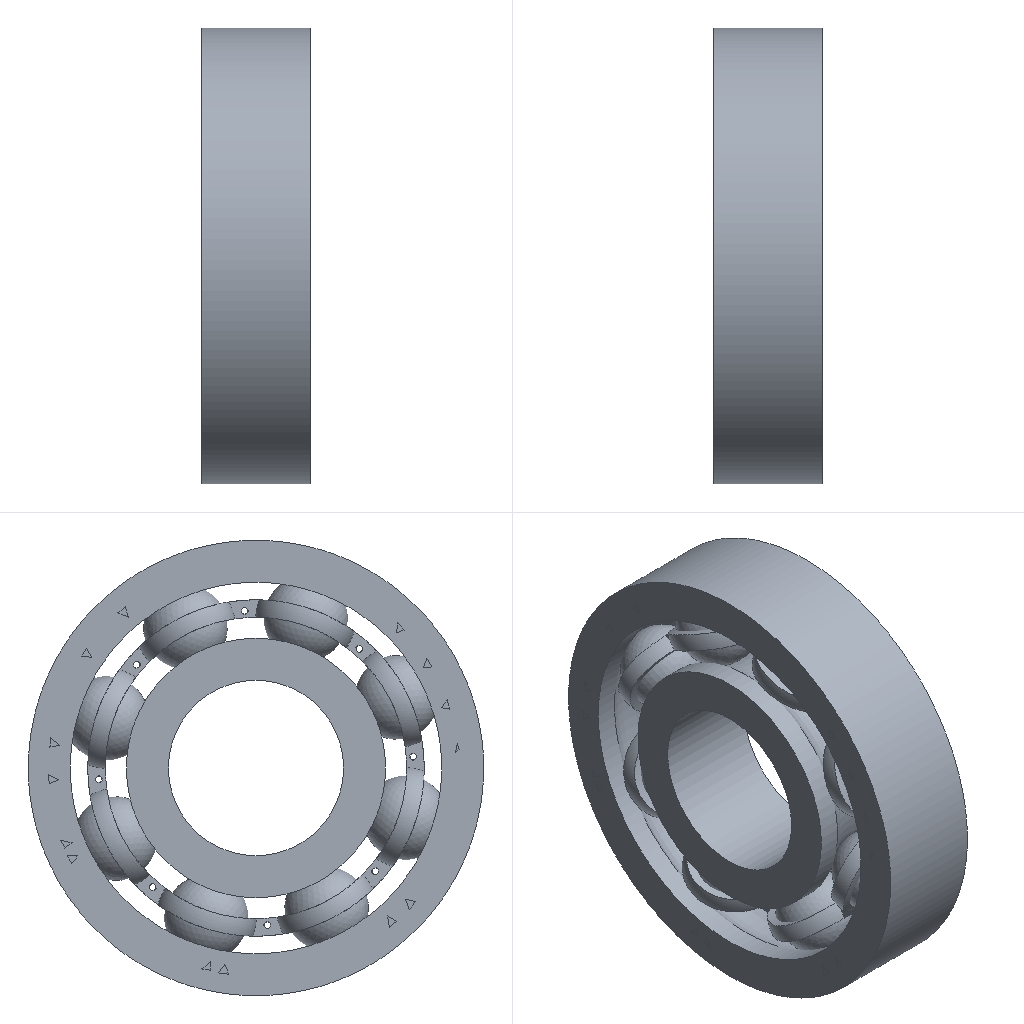Simulation study | ansys workbench
Set-up summary:
category,name,step,type,value,unit,region
solver,ansys_workbench
units,SI m-kg-s (Pa),,stated,"/units,MKS"
analysis,LS1,,static
load_step,LS1,LS1,static,nsubst=1; time=1
mesh,nodes,,,291728
mesh,elements,,,199572
element_type,SOLID187,,,151094
element_type,TARGE170,,,18876
element_type,CONTA174,,,18876
element_type,SOLID186,,,10416
element_type,SURF154,,,310
material,Structural Steel,,E,2e+11,Pa
material,Structural Steel,,nu,0.3
material,Structural Steel,,density,7850,kg m^-3
material,Structural Steel,,conductivity,60.5,W m^-1 C^-1
material,Structural Steel,,specific_heat,434,J kg^-1 C^-1
material,Structural Steel,,cte,1.2e-05,C^-1
material,Structural Steel,,permeability,10000
material,Structural Steel,,resistivity,1.7e-07,kg m^3 A^-2 s^-3
load,Define Force Using Surface Effect Elements,LS1,surface-effect pres face 1,-17113.4,,SURF154 #79
bc,Fixed Supports,model,fixed,[dofs=ALL],,_FIXEDSU
contact,Contact Region,,bonded (always),element=CONTA174
contact,Contact Region 2,,bonded (always),element=CONTA174
contact,Contact Region 3,,bonded (always),element=CONTA174
contact,Contact Region 4,,bonded (always),element=CONTA174
contact,Contact Region 5,,bonded (always),element=CONTA174
contact,Contact Region 6,,bonded (always),element=CONTA174
contact,Contact Region 7,,bonded (always),element=CONTA174
contact,Contact Region 8,,bonded (always),element=CONTA174
contact,Contact Region 9,,bonded (always),element=CONTA174
contact,Contact Region 10,,bonded (always),element=CONTA174
contact,Contact Region 11,,bonded (always),element=CONTA174
contact,Contact Region 12,,bonded (always),element=CONTA174
contact,Contact Region 21,,bonded (always),element=CONTA174
contact,Contact Region 22,,bonded (always),element=CONTA174
contact,Contact Region 23,,bonded (always),element=CONTA174
contact,Contact Region 24,,bonded (always),element=CONTA174
contact,Contact Region 25,,bonded (always),element=CONTA174
contact,Contact Region 26,,bonded (always),element=CONTA174
contact,Contact Region 27,,bonded (always),element=CONTA174
contact,Contact Region 28,,bonded (always),element=CONTA174
contact,Contact Region 29,,bonded (always),element=CONTA174
contact,Contact Region 30,,bonded (always),element=CONTA174
contact,Contact Region 31,,bonded (always),element=CONTA174
contact,Contact Region 32,,bonded (always),element=CONTA174
contact,Contact Region 33,,bonded (always),element=CONTA174
contact,Contact Region 34,,bonded (always),element=CONTA174
contact,Contact Region 35,,bonded (always),element=CONTA174
contact,Contact Region 36,,bonded (always),element=CONTA174
contact,Contact Region 39,,bonded (always),element=CONTA174
contact,Contact Region 40,,bonded (always),element=CONTA174
contact,Contact Region 41,,bonded (always),element=CONTA174
contact,Contact Region 42,,bonded (always),element=CONTA174
contact,Contact Region 43,,bonded (always),element=CONTA174
named_set,_FIXEDSU,,node,1910
Ansys APDL input file, long lists of numbers shortened:
/batch
/config,noeldb,1     ! force off writing results to database
*get,_wallstrt,active,,time,wall
! ANSYS input file written by Workbench version 2024 R2
! File used for geometry attach:
/title,wbnew--____ (A5)
! ****** Begin Custom Load Command Snippet ******
/COM, ACT Extensions:
/COM,     LSDYNA, 2024.2
/COM,/COM,     ANSYSMotion, 2024.2
/COM,
! ****** End   Custom Load Command Snippet ******
*DIM,_wb_ProjectScratch_dir,string,248
_wb_ProjectScratch_dir(1) = ''
*DIM,_wb_SolverFiles_dir,string,248
_wb_SolverFiles_dir(1) = ''
*DIM,_wb_userfiles_dir,string,248
_wb_userfiles_dir(1) = ''
/com,--- Data in consistent MKS units. See Solving Units in the help system for more information.
/units,MKS
/nopr
/wb,file,start              !  signify a WB generated input file
/prep7
! Turn off shape checking because checks already performed inside WB mesher.
! See help system for more information.
SHPP,OFF,,NOWARN
/nolist
etcon,set             ! allow ANSYS to choose best KEYOP's for 180x elements, resets any applicable keyopt to MAPDL defaults
/com,*********** Nodes for the whole assembly ***********
nblock,3,,320900
(1i9,3e20.9e3)
        1     7.105415696E-02    -1.310212572E-01    -3.338176666E-02
! (291727 more lines like these left out)
-1
/wb,elem,start            !  set before creation of elements
/com,*********** Elements for Body 1 'ball 3|Revolve1' ***********
et,1,187
eblock,19,solid,,8093
(19i9)
        1        1        1        1        0        0        0        0       10        0        1      749      951     1669     1661     6914     8412     6923     6922
! (16185 more lines like these left out)
-1
/com,*********** Elements for Body 2 'cage 4|CirPattern2' ***********
et,2,187
eblock,19,solid,,43175
(19i9)
        2        2        2        2        0        0        0        0       10        0     8094    18166    18230    18232    23065    62092    62544    62093    62097
! (86349 more lines like these left out)
-1
/com,*********** Elements for Body 3 'inner ring 2|Revolve1' ***********
et,3,186
keyo,3,2,1          ! set full integration on SOLID186
eblock,19,solid,,3720
(19i9)
        3        3        3        3        0        0        0        0       20        0    51269    84215    84416    84251    84417    87104    86903    87068    86902
! (7439 more lines like these left out)
-1
/com,*********** Elements for Body 4 'outer ring 1|Revolve2' ***********
et,4,186
keyo,4,2,1          ! set full integration on SOLID186
eblock,19,solid,,6696
(19i9)
        4        4        4        4        0        0        0        0       20        0    54989   102514   102900   102901   102546   107625   107239   107238   107593
! (13391 more lines like these left out)
-1
/com,*********** Elements for Body 5 'ball 3|Revolve1[2]' ***********
et,5,187
eblock,19,solid,,8093
(19i9)
        5        5        5        5        0        0        0        0       10        0    61685   136204   136406   137124   137116   142369   143867   142378   142377
! (16185 more lines like these left out)
-1
/com,*********** Elements for Body 6 'ball 3|Revolve1[3]' ***********
et,6,187
eblock,19,solid,,8093
(19i9)
        6        6        6        6        0        0        0        0       10        0    69778   148217   148419   149137   149129   154382   155880   154391   154390
! (16185 more lines like these left out)
-1
/com,*********** Elements for Body 7 'ball 3|Revolve1[4]' ***********
et,7,187
eblock,19,solid,,8093
(19i9)
        7        7        7        7        0        0        0        0       10        0    77871   160230   160432   161150   161142   166395   167893   166404   166403
! (16185 more lines like these left out)
-1
/com,*********** Elements for Body 8 'ball 3|Revolve1[5]' ***********
et,8,187
eblock,19,solid,,8093
(19i9)
        8        8        8        8        0        0        0        0       10        0    85964   172243   172445   173163   173155   178408   179906   178417   178416
! (16185 more lines like these left out)
-1
/com,*********** Elements for Body 9 'ball 3|Revolve1[6]' ***********
et,9,187
eblock,19,solid,,8093
(19i9)
        9        9        9        9        0        0        0        0       10        0    94057   184256   184458   185176   185168   190421   191919   190430   190429
! (16185 more lines like these left out)
-1
! (2 more sections like these left out)
/com,*********** Elements for Body 12 'cage 4|CirPattern2[2]' ***********
et,12,187
eblock,19,solid,,43175
(19i9)
       12       12       12       12        0        0        0        0       10        0   118336   225699   225763   225765   230598   269625   270077   269626   269630
! (86349 more lines like these left out)
-1
/wb,elem,end               !  done creating elements
/com,*********** Send User Defined Coordinate System(s) ***********
csys,0
toffst,273.15,      ! Temperature offset from absolute zero
/com,*********** Set Reference Temperature ***********
tref,22.
/wb,mat,start              !  starting to send materials
/com,*********** Send Materials ***********
Temperature = 'TEMP' ! Temperature
MP,DENS,1,7850,	! kg m^-3
MP,ALPX,1,1.2e-05,	! C^-1
MP,C,1,434,	! J kg^-1 C^-1
MP,KXX,1,60.5,	! W m^-1 C^-1
MP,RSVX,1,1.7e-07,	! kg m^3 A^-2 s^-3
MP,EX,1,200000000000,	! Pa
MP,NUXY,1,0.3,
MP,MURX,1,10000,
Temperature = 'TEMP' ! Temperature
MP,DENS,2,7850,	! kg m^-3
MP,ALPX,2,1.2e-05,	! C^-1
MP,C,2,434,	! J kg^-1 C^-1
MP,KXX,2,60.5,	! W m^-1 C^-1
MP,RSVX,2,1.7e-07,	! kg m^3 A^-2 s^-3
MP,EX,2,200000000000,	! Pa
MP,NUXY,2,0.3,
MP,MURX,2,10000,
Temperature = 'TEMP' ! Temperature
MP,DENS,3,7850,	! kg m^-3
MP,ALPX,3,1.2e-05,	! C^-1
MP,C,3,434,	! J kg^-1 C^-1
MP,KXX,3,60.5,	! W m^-1 C^-1
MP,RSVX,3,1.7e-07,	! kg m^3 A^-2 s^-3
MP,EX,3,200000000000,	! Pa
MP,NUXY,3,0.3,
MP,MURX,3,10000,
Temperature = 'TEMP' ! Temperature
MP,DENS,4,7850,	! kg m^-3
MP,ALPX,4,1.2e-05,	! C^-1
MP,C,4,434,	! J kg^-1 C^-1
MP,KXX,4,60.5,	! W m^-1 C^-1
MP,RSVX,4,1.7e-07,	! kg m^3 A^-2 s^-3
MP,EX,4,200000000000,	! Pa
MP,NUXY,4,0.3,
MP,MURX,4,10000,
Temperature = 'TEMP' ! Temperature
MP,DENS,5,7850,	! kg m^-3
MP,ALPX,5,1.2e-05,	! C^-1
MP,C,5,434,	! J kg^-1 C^-1
MP,KXX,5,60.5,	! W m^-1 C^-1
MP,RSVX,5,1.7e-07,	! kg m^3 A^-2 s^-3
MP,EX,5,200000000000,	! Pa
MP,NUXY,5,0.3,
MP,MURX,5,10000,
Temperature = 'TEMP' ! Temperature
MP,DENS,6,7850,	! kg m^-3
MP,ALPX,6,1.2e-05,	! C^-1
MP,C,6,434,	! J kg^-1 C^-1
MP,KXX,6,60.5,	! W m^-1 C^-1
MP,RSVX,6,1.7e-07,	! kg m^3 A^-2 s^-3
MP,EX,6,200000000000,	! Pa
MP,NUXY,6,0.3,
MP,MURX,6,10000,
Temperature = 'TEMP' ! Temperature
MP,DENS,7,7850,	! kg m^-3
MP,ALPX,7,1.2e-05,	! C^-1
MP,C,7,434,	! J kg^-1 C^-1
MP,KXX,7,60.5,	! W m^-1 C^-1
MP,RSVX,7,1.7e-07,	! kg m^3 A^-2 s^-3
MP,EX,7,200000000000,	! Pa
MP,NUXY,7,0.3,
MP,MURX,7,10000,
Temperature = 'TEMP' ! Temperature
MP,DENS,8,7850,	! kg m^-3
MP,ALPX,8,1.2e-05,	! C^-1
MP,C,8,434,	! J kg^-1 C^-1
MP,KXX,8,60.5,	! W m^-1 C^-1
MP,RSVX,8,1.7e-07,	! kg m^3 A^-2 s^-3
MP,EX,8,200000000000,	! Pa
MP,NUXY,8,0.3,
MP,MURX,8,10000,
Temperature = 'TEMP' ! Temperature
MP,DENS,9,7850,	! kg m^-3
MP,ALPX,9,1.2e-05,	! C^-1
MP,C,9,434,	! J kg^-1 C^-1
MP,KXX,9,60.5,	! W m^-1 C^-1
MP,RSVX,9,1.7e-07,	! kg m^3 A^-2 s^-3
MP,EX,9,200000000000,	! Pa
MP,NUXY,9,0.3,
MP,MURX,9,10000,
Temperature = 'TEMP' ! Temperature
MP,DENS,10,7850,	! kg m^-3
MP,ALPX,10,1.2e-05,	! C^-1
MP,C,10,434,	! J kg^-1 C^-1
MP,KXX,10,60.5,	! W m^-1 C^-1
MP,RSVX,10,1.7e-07,	! kg m^3 A^-2 s^-3
MP,EX,10,200000000000,	! Pa
MP,NUXY,10,0.3,
MP,MURX,10,10000,
Temperature = 'TEMP' ! Temperature
MP,DENS,11,7850,	! kg m^-3
MP,ALPX,11,1.2e-05,	! C^-1
MP,C,11,434,	! J kg^-1 C^-1
MP,KXX,11,60.5,	! W m^-1 C^-1
MP,RSVX,11,1.7e-07,	! kg m^3 A^-2 s^-3
MP,EX,11,200000000000,	! Pa
MP,NUXY,11,0.3,
MP,MURX,11,10000,
Temperature = 'TEMP' ! Temperature
MP,DENS,12,7850,	! kg m^-3
MP,ALPX,12,1.2e-05,	! C^-1
MP,C,12,434,	! J kg^-1 C^-1
MP,KXX,12,60.5,	! W m^-1 C^-1
MP,RSVX,12,1.7e-07,	! kg m^3 A^-2 s^-3
MP,EX,12,200000000000,	! Pa
MP,NUXY,12,0.3,
MP,MURX,12,10000,
/wb,mat,end                !  done sending materials
!************************* Model Summary ********************
!ball 3|Revolve1,	ç»æé¢,	matid,	1
!cage 4|CirPattern2,	ç»æé¢,	matid,	2
!inner ring 2|Revolve1,	ç»æé¢,	matid,	3
!outer ring 1|Revolve2,	ç»æé¢,	matid,	4
!ball 3|Revolve1[2],	ç»æé¢,	matid,	5
!ball 3|Revolve1[3],	ç»æé¢,	matid,	6
!ball 3|Revolve1[4],	ç»æé¢,	matid,	7
!ball 3|Revolve1[5],	ç»æé¢,	matid,	8
!ball 3|Revolve1[6],	ç»æé¢,	matid,	9
!ball 3|Revolve1[7],	ç»æé¢,	matid,	10
!ball 3|Revolve1[8],	ç»æé¢,	matid,	11
!cage 4|CirPattern2[2],	ç»æé¢,	matid,	12
!************************* End Model Summary ********************
! get the diagonal of the bounding box. Needed later for other things
*get,_xmin,node,,mnloc,x
*get,_ymin,node,,mnloc,y
*get,_zmin,node,,mnloc,z
*get,_xmax,node,,mxloc,x
*get,_ymax,node,,mxloc,y
*get,_zmax,node,,mxloc,z
_ASMDIAG=(_xmax-_xmin)*(_xmax-_xmin)+(_ymax-_ymin)*(_ymax-_ymin)+(_zmax-_zmin)*(_zmax-_zmin)
_ASMDIAG=SQRT(_ASMDIAG)
/wb,contact,start          !  starting to send contact
/com,*********** Create Contact "½Ó´¥ÇøÓò" ***********
/com,            Real Constant Set For Above Contact Is 14 & 13
*set,tid,14
*set,cid,13
r,tid
r,cid
et,tid,170
et,cid,174
eblock,10,,,275
(15i9)
   204739       14       14       14        0       36       37      315      315     1973     1985      315     1976
! (274 more lines like these left out)
-1
eblock,10,,,275
(15i9)
   205014       13       13       13        0       36       37      315      315     1973     1985      315     1976
! (274 more lines like these left out)
-1
eblock,10,,,440
(15i9)
   205289       13       14       13        0    13834    13833    18365    18365    34711    34715    18365    34721
! (439 more lines like these left out)
-1
eblock,10,,,440
(15i9)
   205729       14       13       14        0    13834    13833    18365    18365    34711    34715    18365    34721
! (439 more lines like these left out)
-1
keyo,cid,8,2               ! auto create asymmetric contact (from Program Controlled setting)
keyo,cid,10,0              ! adjust contact stiffness each NR iteration (from Program Controlled setting)
keyo,cid,12,5              ! bonded always
keyo,cid,18,1              ! small sliding turned on by application
keyo,cid,2,2               ! MPC for bonded contacts (from Program Controlled setting)
keyo,tid,5,0               ! Automatic constraint type detection
keyo,cid,4,2               ! on nodal point - normal to target surface (from Program Controlled setting)
keyo,cid,9,1               ! ignore initial gaps/penetration
keyo,cid,7,0               ! No Prediction
rmod,tid,3,10.      ! FKN
rmod,tid,5,0.       ! ICONT
rmod,tid,6,0.       ! PINB
rmod,tid,10,0.      ! CNOF
rmod,tid,12,0.      ! FKT
rmod,tid,36,101     ! WB DSID
rmod,cid,3,10.      ! FKN
rmod,cid,5,0.       ! ICONT
rmod,cid,6,0.       ! PINB
rmod,cid,10,0.      ! CNOF
rmod,cid,12,0.      ! FKT
rmod,cid,36,101     ! WB DSID
/com,*********** Create Contact "½Ó´¥ÇøÓò 2" ***********
/com,            Real Constant Set For Above Contact Is 16 & 15
*set,tid,16
*set,cid,15
r,tid
r,cid
et,tid,170
et,cid,174
eblock,10,,,200
(15i9)
   206169       16       16       16        0       15       14      326      326     1784     1787      326     1796
! (199 more lines like these left out)
-1
eblock,10,,,200
(15i9)
   206369       15       15       15        0       15       14      326      326     1784     1787      326     1796
! (199 more lines like these left out)
-1
eblock,10,,,44
(15i9)
   206569       15       16       15        0    88393    88394    88356    88355   101291   101217   101214   101215
! (43 more lines like these left out)
-1
eblock,10,,,44
(15i9)
   206613       16       15       16        0    88393    88394    88356    88355   101291   101217   101214   101215
! (43 more lines like these left out)
-1
keyo,cid,8,2               ! auto create asymmetric contact (from Program Controlled setting)
keyo,cid,10,0              ! adjust contact stiffness each NR iteration (from Program Controlled setting)
keyo,cid,12,5              ! bonded always
keyo,cid,18,1              ! small sliding turned on by application
keyo,cid,2,2               ! MPC for bonded contacts (from Program Controlled setting)
keyo,tid,5,0               ! Automatic constraint type detection
keyo,cid,4,2               ! on nodal point - normal to target surface (from Program Controlled setting)
keyo,cid,9,1               ! ignore initial gaps/penetration
keyo,cid,7,0               ! No Prediction
rmod,tid,3,10.      ! FKN
rmod,tid,5,0.       ! ICONT
rmod,tid,6,0.       ! PINB
rmod,tid,10,0.      ! CNOF
rmod,tid,12,0.      ! FKT
rmod,tid,36,104     ! WB DSID
rmod,cid,3,10.      ! FKN
rmod,cid,5,0.       ! ICONT
rmod,cid,6,0.       ! PINB
rmod,cid,10,0.      ! CNOF
rmod,cid,12,0.      ! FKT
rmod,cid,36,104     ! WB DSID
/com,*********** Create Contact "½Ó´¥ÇøÓò 3" ***********
/com,            Real Constant Set For Above Contact Is 18 & 17
*set,tid,18
*set,cid,17
r,tid
r,cid
et,tid,170
et,cid,174
eblock,10,,,314
(15i9)
   206657       18       18       18        0       32       33      327      327     1939     1951      327     1942
! (313 more lines like these left out)
-1
eblock,10,,,314
(15i9)
   206971       17       17       17        0       32       33      327      327     1939     1951      327     1942
! (313 more lines like these left out)
-1
eblock,10,,,61
(15i9)
   207285       17       18       17        0   108434   108435   108396   108397   129973   129898   129897   129900
! (60 more lines like these left out)
-1
eblock,10,,,61
(15i9)
   207346       18       17       18        0   108434   108435   108396   108397   129973   129898   129897   129900
! (60 more lines like these left out)
-1
keyo,cid,8,2               ! auto create asymmetric contact (from Program Controlled setting)
keyo,cid,10,0              ! adjust contact stiffness each NR iteration (from Program Controlled setting)
keyo,cid,12,5              ! bonded always
keyo,cid,18,1              ! small sliding turned on by application
keyo,cid,2,2               ! MPC for bonded contacts (from Program Controlled setting)
keyo,tid,5,0               ! Automatic constraint type detection
keyo,cid,4,2               ! on nodal point - normal to target surface (from Program Controlled setting)
keyo,cid,9,1               ! ignore initial gaps/penetration
keyo,cid,7,0               ! No Prediction
rmod,tid,3,10.      ! FKN
rmod,tid,5,0.       ! ICONT
rmod,tid,6,0.       ! PINB
rmod,tid,10,0.      ! CNOF
rmod,tid,12,0.      ! FKT
rmod,tid,36,107     ! WB DSID
rmod,cid,3,10.      ! FKN
rmod,cid,5,0.       ! ICONT
rmod,cid,6,0.       ! PINB
rmod,cid,10,0.      ! CNOF
rmod,cid,12,0.      ! FKT
rmod,cid,36,107     ! WB DSID
/com,*********** Create Contact "½Ó´¥ÇøÓò 4" ***********
/com,            Real Constant Set For Above Contact Is 20 & 19
*set,tid,20
*set,cid,19
r,tid
r,cid
et,tid,170
et,cid,174
eblock,10,,,265
(15i9)
   207407       20       20       20        0        3        1      335      335     1670     1674      335     1693
! (264 more lines like these left out)
-1
eblock,10,,,265
(15i9)
   207672       19       19       19        0        3        1      335      335     1670     1674      335     1693
! (264 more lines like these left out)
-1
eblock,10,,,440
(15i9)
   207937       19       20       19        0   221380   221379   225826   225826   242347   242350   225826   242357
! (439 more lines like these left out)
-1
eblock,10,,,440
(15i9)
   208377       20       19       20        0   221380   221379   225826   225826   242347   242350   225826   242357
! (439 more lines like these left out)
-1
keyo,cid,8,2               ! auto create asymmetric contact (from Program Controlled setting)
keyo,cid,10,0              ! adjust contact stiffness each NR iteration (from Program Controlled setting)
keyo,cid,12,5              ! bonded always
keyo,cid,18,1              ! small sliding turned on by application
keyo,cid,2,2               ! MPC for bonded contacts (from Program Controlled setting)
keyo,tid,5,0               ! Automatic constraint type detection
keyo,cid,4,2               ! on nodal point - normal to target surface (from Program Controlled setting)
keyo,cid,9,1               ! ignore initial gaps/penetration
keyo,cid,7,0               ! No Prediction
rmod,tid,3,10.      ! FKN
rmod,tid,5,0.       ! ICONT
rmod,tid,6,0.       ! PINB
rmod,tid,10,0.      ! CNOF
rmod,tid,12,0.      ! FKT
rmod,tid,36,110     ! WB DSID
rmod,cid,3,10.      ! FKN
rmod,cid,5,0.       ! ICONT
rmod,cid,6,0.       ! PINB
rmod,cid,10,0.      ! CNOF
rmod,cid,12,0.      ! FKT
rmod,cid,36,110     ! WB DSID
/com,*********** Create Contact "½Ó´¥ÇøÓò 5" ***********
/com,            Real Constant Set For Above Contact Is 22 & 21
*set,tid,22
*set,cid,21
r,tid
r,cid
et,tid,170
et,cid,174
eblock,10,,,460
(15i9)
   208817       22       22       22        0    12128    12126    12130    12130    23957    23958    12130    23971
! (459 more lines like these left out)
-1
eblock,10,,,460
(15i9)
   209277       21       21       21        0    12128    12126    12130    12130    23957    23958    12130    23971
! (459 more lines like these left out)
-1
eblock,10,,,285
(15i9)
   209737       21       22       21        0   135491   135492   135770   135770   137428   137440   135770   137431
! (284 more lines like these left out)
-1
eblock,10,,,285
(15i9)
   210022       22       21       22        0   135491   135492   135770   135770   137428   137440   135770   137431
! (284 more lines like these left out)
-1
keyo,cid,8,2               ! auto create asymmetric contact (from Program Controlled setting)
keyo,cid,10,0              ! adjust contact stiffness each NR iteration (from Program Controlled setting)
keyo,cid,12,5              ! bonded always
keyo,cid,18,1              ! small sliding turned on by application
keyo,cid,2,2               ! MPC for bonded contacts (from Program Controlled setting)
keyo,tid,5,0               ! Automatic constraint type detection
keyo,cid,4,2               ! on nodal point - normal to target surface (from Program Controlled setting)
keyo,cid,9,1               ! ignore initial gaps/penetration
keyo,cid,7,0               ! No Prediction
rmod,tid,3,10.      ! FKN
rmod,tid,5,0.       ! ICONT
rmod,tid,6,0.       ! PINB
rmod,tid,10,0.      ! CNOF
rmod,tid,12,0.      ! FKT
rmod,tid,36,113     ! WB DSID
rmod,cid,3,10.      ! FKN
rmod,cid,5,0.       ! ICONT
rmod,cid,6,0.       ! PINB
rmod,cid,10,0.      ! CNOF
rmod,cid,12,0.      ! FKT
rmod,cid,36,113     ! WB DSID
! (28 more sections like these left out)
/wb,contact,end            !  done creating contacts
/golist
/wb,load,start             !  starting to send loads
/com,*********** Fixed Supports ***********
CMBLOCK,_FIXEDSU,NODE,     1910
(8i10)
    107626    107627    107628    107629    107630    107631    107632    107633
! (238 more lines like these left out)
cmsel,s,_FIXEDSU
d,all,all
nsel,all
/com,*********** Define Force Using Surface Effect Elements ***********
local,12,0,0.,0.,0.,0.,0.,0.
csys,0
et,79,154
mat,79
eblock,10,,,310
(15i9)
   242491       79       79       79       12    87344    87143    87345    87179    98722    98723    98841    98840
! (309 more lines like these left out)
-1
esel,s,type,,79
keyop,79,2,1        ! Apply load in local coordinate system
keyop,79,7,1        ! Use original area so load is constant in large deformation
esel,all
/gst,on,on
fini
*get,_numnode,node,0,count
*get,_numelem,elem,0,count
*get, _MAXELEMNUM, elem, 0, NUM, MAX
*get, _MAXNODENUM, node, 0, NUM, MAX
*get, _MAXELEMTYPE, etyp, 0, NUM, MAX
*get, _MAXREALCONST, rcon, 0, NUM, MAX
/go
/wb,load,end               !  done creating loads
/com,--- Number of total nodes = %_numnode%
/com,--- Number of contact elements = 38062
/com,--- Number of spring elements = 0
/com,--- Number of bearing elements = 0
/com,--- Number of solid elements = 161510
/com,--- Number of condensed parts = 0
/com,--- Number of total elements = %_numelem%
*get,_wallbsol,active,,time,wall
/com,****************************************************************************
/com,*************************    SOLUTION       ********************************
/com,****************************************************************************
/solu
antype,0                   ! static analysis
_thickRatio=  1     ! Ratio of thick parts in the model
eqsl,pcg,1e-8,,,,,,1
cntr,print,1               ! print out contact info and also make no initial contact an error
dmpoption,emat,no             ! Don't combine emat file for DANSYS
dmpoption,esav,no             ! Don't combine esav file for DANSYS
nldiag,cont,iter           ! print out contact info each equilibrium iteration
rescontrol,,none                 ! Do not keep any restart files
/com,****************************************************
/com,******************* SOLVE FOR LS 1 OF 1 ****************
esel,s,type,,79
nsle
sfe,all,1,pres,1,-17113.432
sfe,all,2,pres,1,0.
sfe,all,3,pres,1,0.
nsel,all
esel,all
/nopr
/gopr
nsub,1,1,1
time,1.
outres,erase
outres,all,none
outres,nsol,all,
outres,rsol,all
outres,eangl,all
outres,etmp,all
outres,veng,all
outres,strs,all,
outres,epel,all,
outres,eppl,all,
outres,cont,all,
! *********** WB SOLVE COMMAND ***********
! check interactive state
*get,ANSINTER_,active,,int
*if,ANSINTER_,ne,0,then
/eof
*endif
solve
/com *************** Write FE CONNECTORS *********
CEWRITE,file,ce,,INTE
/com,****************************************************
/com,*************** FINISHED SOLVE FOR LS 1 *************
*get,_wallasol,active,,time,wall
/nopr
*get,_numnode,node,0,count
*get,_numelem,elem,0,count
*get, _MAXELEMNUM, elem, 0, NUM, MAX
*get, _MAXNODENUM, node, 0, NUM, MAX,,,INTERNAL
*get, _MAXELEMTYPE, etyp, 0, NUM, MAX
*get, _MAXREALCONST, rcon, 0, NUM, MAX
*get,_NSOLTHREADS,active,0,ntfs
*get,_NSOLPROCESSES,active,0,npfs
/gopr
*get,_PCGITER,active,,solu,cgiter
/post1
xmlo,ENCODING,ISO-8859-1
xmlo,parm
/xml,parm,xml
fini
/gopr
*get,_walldone,active,,time,wall
_preptime=(_wallbsol-_wallstrt)*3600
_solvtime=(_wallasol-_wallbsol)*3600
_posttime=(_walldone-_wallasol)*3600
_totaltim=(_walldone-_wallstrt)*3600
*get,_dlbratio,active,0,solu,dlbr
*get,_combtime,active,0,solu,comb
*get,_ssmode,active,0,solu,ssmm
*get,_ndofs,active,0,solu,ndof
*get,_sol_end_time,active,0,set,time
*if,_sol_end_time,eq,1.,then
/fclean				!clean distributed files
*endif
/com,--- Total number of nodes = %_numnode%
/com,--- Total number of elements = %_numelem%
/com,--- Element load balance ratio = %_dlbratio%
/com,--- Time to combine distributed files = %_combtime%
/com,--- Sparse memory mode = %_ssmode%
/com,--- Number of DOF = %_ndofs%
/wb,file,end               ! done with WB generated input
Results summary:
result,analyses[0].index,,,1
result,analyses[0].system,,,SYS
result,analyses[0].deck,,,deck.dat
result,analyses[0].solve_status,,,completed
result,analyses[0].analysis_type,,,static
result,analyses[0].physics,,,mechanical
result,analyses[0].unit_system,,,"MKS: m, kg, N, s, V, A, degC"
result,analyses[0].n_sets,,,1
result,analyses[0].load_steps[0].set,set=1,,1
result,analyses[0].load_steps[0].time_or_freq,set=1,,1
result,analyses[0].load_steps[0].max_displacement_magnitude,set=1,,2.77398e-08
result,analyses[0].load_steps[0].max_von_mises_nodal,set=1,,246419
result,analyses[0].load_steps[0].reaction_force_sum_xyz[1],set=1,,40
result,analyses[0].load_steps[0].reaction_force_sum_xyz[2],set=1,,-8.58629e-10
result,analyses[0].load_steps[0].reaction_force_sum_xyz[3],set=1,,-6.00602e-09